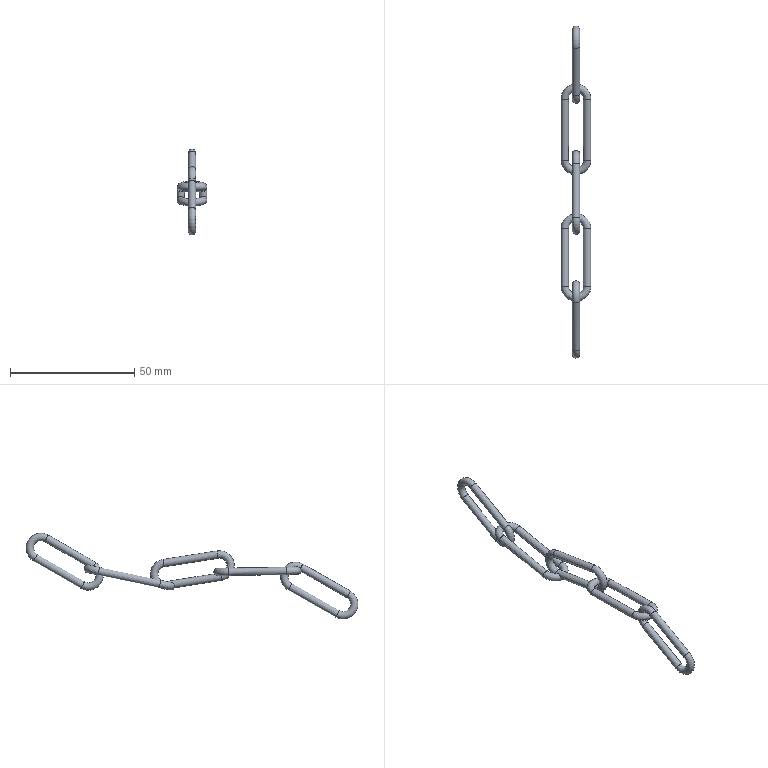Part | NX | features ACO1606-1-04.4 2 | 1 solid | 22 faces | box 12 x 133.567 x 34.55 mm | volume 2590 mm3 | cylinder 12 | torus 10 | commonest cylinder face diameters 3 x12
STEP:
#1=CARTESIAN_POINT('',(-1014.667,-666.313,-187.929));
#2=VERTEX_POINT('',#1);
#3=CARTESIAN_POINT('',(-1013.167,-665.571,-189.232));
#4=VERTEX_POINT('',#3);
#5=CARTESIAN_POINT('',(-1014.667,-665.571,-189.232));
#6=DIRECTION('',(0.,0.8691,0.4946));
#7=DIRECTION('',(1.,0.,0.));
#8=AXIS2_PLACEMENT_3D('',#5,#6,#7);
#9=CIRCLE('',#8,1.5);
#10=EDGE_CURVE('',#2,#4,#9,.T.);
#11=ORIENTED_EDGE('',*,*,#10,.T.);
#12=CARTESIAN_POINT('',(-1014.667,-664.829,-190.536));
#13=VERTEX_POINT('',#12);
#14=CARTESIAN_POINT('',(-1014.667,-665.571,-189.232));
#15=DIRECTION('',(0.,0.8691,0.4946));
#16=DIRECTION('',(1.,0.,0.));
#17=AXIS2_PLACEMENT_3D('',#14,#15,#16);
#18=CIRCLE('',#17,1.5);
#19=EDGE_CURVE('',#4,#13,#18,.T.);
#20=ORIENTED_EDGE('',*,*,#19,.T.);
#21=CARTESIAN_POINT('',(-1016.167,-665.571,-189.232));
#22=VERTEX_POINT('',#21);
#23=CARTESIAN_POINT('',(-1014.667,-665.571,-189.232));
#24=DIRECTION('',(0.,0.8691,0.4946));
#25=DIRECTION('',(1.,0.,0.));
#26=AXIS2_PLACEMENT_3D('',#23,#24,#25);
#27=CIRCLE('',#26,1.5);
#28=EDGE_CURVE('',#13,#22,#27,.T.);
#29=ORIENTED_EDGE('',*,*,#28,.T.);
#30=CARTESIAN_POINT('',(-1014.667,-665.571,-189.232));
#31=DIRECTION('',(0.,0.8691,0.4946));
#32=DIRECTION('',(1.,0.,0.));
#33=AXIS2_PLACEMENT_3D('',#30,#31,#32);
#34=CIRCLE('',#33,1.5);
#35=EDGE_CURVE('',#22,#2,#34,.T.);
#36=ORIENTED_EDGE('',*,*,#35,.T.);
#37=EDGE_LOOP('',(#11,#20,#29,#36));
#38=FACE_BOUND('',#37,.T.);
#39=CARTESIAN_POINT('',(-1013.333,-669.683,-182.007));
#40=VERTEX_POINT('',#39);
#41=CARTESIAN_POINT('',(-1014.667,-670.765,-180.107));
#42=VERTEX_POINT('',#41);
#43=CARTESIAN_POINT('',(-1014.667,-670.023,-181.41));
#44=DIRECTION('',(0.,-0.8691,-0.4946));
#45=DIRECTION('',(1.,0.,0.));
#46=AXIS2_PLACEMENT_3D('',#43,#44,#45);
#47=CIRCLE('',#46,1.5);
#48=EDGE_CURVE('',#40,#42,#47,.T.);
#49=ORIENTED_EDGE('',*,*,#48,.F.);
#50=CARTESIAN_POINT('',(-1016.001,-669.683,-182.007));
#51=VERTEX_POINT('',#50);
#52=CARTESIAN_POINT('',(-1013.333,-669.683,-182.007));
#53=CARTESIAN_POINT('',(-1013.251,-669.485,-181.709));
#54=CARTESIAN_POINT('',(-1013.206,-668.885,-181.238));
#55=CARTESIAN_POINT('',(-1013.224,-667.927,-181.234));
#56=CARTESIAN_POINT('',(-1013.353,-667.283,-181.603));
#57=CARTESIAN_POINT('',(-1013.736,-666.964,-182.19));
#58=CARTESIAN_POINT('',(-1014.663,-667.168,-182.548));
#59=CARTESIAN_POINT('',(-1015.587,-666.965,-182.199));
#60=CARTESIAN_POINT('',(-1015.978,-667.275,-181.609));
#61=CARTESIAN_POINT('',(-1016.11,-667.918,-181.235));
#62=CARTESIAN_POINT('',(-1016.128,-668.884,-181.237));
#63=CARTESIAN_POINT('',(-1016.084,-669.485,-181.709));
#64=CARTESIAN_POINT('',(-1016.001,-669.683,-182.007));
#65=B_SPLINE_CURVE_WITH_KNOTS('',3,(#52,#53,#54,#55,#56,#57,#58,#59,#60,#61,#62,#63,#64),.UNSPECIFIED.,.F.,.F.,(4,1,1,1,1,1,1,1,1,1,4),(0.,0.001085,0.002169,0.002711,0.003254,0.004338,0.005423,0.005965,0.006507,0.007592,0.008676),.UNSPECIFIED.);
#66=EDGE_CURVE('',#40,#51,#65,.T.);
#67=ORIENTED_EDGE('',*,*,#66,.T.);
#68=CARTESIAN_POINT('',(-1016.167,-670.023,-181.41));
#69=VERTEX_POINT('',#68);
#70=CARTESIAN_POINT('',(-1014.667,-670.023,-181.41));
#71=DIRECTION('',(0.,-0.8691,-0.4946));
#72=DIRECTION('',(1.,0.,0.));
#73=AXIS2_PLACEMENT_3D('',#70,#71,#72);
#74=CIRCLE('',#73,1.5);
#75=EDGE_CURVE('',#69,#51,#74,.T.);
#76=ORIENTED_EDGE('',*,*,#75,.F.);
#77=CARTESIAN_POINT('',(-1014.667,-670.023,-181.41));
#78=DIRECTION('',(0.,-0.8691,-0.4946));
#79=DIRECTION('',(1.,0.,0.));
#80=AXIS2_PLACEMENT_3D('',#77,#78,#79);
#81=CIRCLE('',#80,1.5);
#82=EDGE_CURVE('',#42,#69,#81,.T.);
#83=ORIENTED_EDGE('',*,*,#82,.F.);
#84=EDGE_LOOP('',(#49,#67,#76,#83));
#85=FACE_BOUND('',#84,.T.);
#86=CARTESIAN_POINT('',(-1014.667,-667.797,-185.321));
#87=DIRECTION('',(1.,0.,0.));
#88=DIRECTION('',(0.,0.,-1.));
#89=AXIS2_PLACEMENT_3D('',#86,#87,#88);
#90=TOROIDAL_SURFACE('',#89,4.5,1.5);
#91=ADVANCED_FACE('',(#38,#85),#90,.T.);
#92=CARTESIAN_POINT('',(-1016.001,-669.683,-182.007));
#93=CARTESIAN_POINT('',(-1015.928,-669.859,-182.27));
#94=CARTESIAN_POINT('',(-1015.636,-670.028,-182.868));
#95=CARTESIAN_POINT('',(-1014.667,-669.985,-183.25));
#96=CARTESIAN_POINT('',(-1013.698,-670.028,-182.868));
#97=CARTESIAN_POINT('',(-1013.406,-669.859,-182.27));
#98=CARTESIAN_POINT('',(-1013.333,-669.683,-182.007));
#99=B_SPLINE_CURVE_WITH_KNOTS('',3,(#92,#93,#94,#95,#96,#97,#98),.UNSPECIFIED.,.F.,.F.,(4,1,1,1,4),(-0.002944,-0.001984,-0.001024,-0.00006463,0.0008951),.UNSPECIFIED.);
#100=EDGE_CURVE('',#51,#40,#99,.T.);
#101=ORIENTED_EDGE('',*,*,#100,.T.);
#102=ORIENTED_EDGE('',*,*,#48,.T.);
#103=ORIENTED_EDGE('',*,*,#82,.T.);
#104=ORIENTED_EDGE('',*,*,#75,.T.);
#105=EDGE_LOOP('',(#101,#102,#103,#104));
#106=FACE_BOUND('',#105,.T.);
#107=CARTESIAN_POINT('',(-1013.167,-689.143,-192.292));
#108=VERTEX_POINT('',#107);
#109=CARTESIAN_POINT('',(-1014.667,-689.143,-192.292));
#110=DIRECTION('',(0.,-0.8691,-0.4946));
#111=DIRECTION('',(1.,0.,0.));
#112=AXIS2_PLACEMENT_3D('',#109,#110,#111);
#113=CIRCLE('',#112,1.5);
#114=EDGE_CURVE('',#108,#108,#113,.T.);
#115=ORIENTED_EDGE('',*,*,#114,.F.);
#116=EDGE_LOOP('',(#115));
#117=FACE_BOUND('',#116,.T.);
#118=CARTESIAN_POINT('',(-1014.667,-678.726,-186.364));
#119=DIRECTION('',(0.,0.8691,0.4946));
#120=DIRECTION('',(0.,0.4946,-0.8691));
#121=AXIS2_PLACEMENT_3D('',#118,#119,#120);
#122=CYLINDRICAL_SURFACE('',#121,1.5);
#123=ADVANCED_FACE('',(#106,#117),#122,.T.);
#124=CARTESIAN_POINT('',(-1013.167,-684.691,-200.114));
#125=VERTEX_POINT('',#124);
#126=CARTESIAN_POINT('',(-1014.667,-684.691,-200.114));
#127=DIRECTION('',(0.,0.8691,0.4946));
#128=DIRECTION('',(1.,0.,0.));
#129=AXIS2_PLACEMENT_3D('',#126,#127,#128);
#130=CIRCLE('',#129,1.5);
#131=EDGE_CURVE('',#125,#125,#130,.T.);
#132=ORIENTED_EDGE('',*,*,#131,.T.);
#133=EDGE_LOOP('',(#132));
#134=FACE_BOUND('',#133,.T.);
#135=ORIENTED_EDGE('',*,*,#19,.F.);
#136=ORIENTED_EDGE('',*,*,#10,.F.);
#137=ORIENTED_EDGE('',*,*,#35,.F.);
#138=ORIENTED_EDGE('',*,*,#28,.F.);
#139=EDGE_LOOP('',(#135,#136,#137,#138));
#140=FACE_BOUND('',#139,.T.);
#141=CARTESIAN_POINT('',(-1014.667,-675.988,-195.161));
#142=DIRECTION('',(0.,-0.8691,-0.4946));
#143=DIRECTION('',(0.,-0.4946,0.8691));
#144=AXIS2_PLACEMENT_3D('',#141,#142,#143);
#145=CYLINDRICAL_SURFACE('',#144,1.5);
#146=ADVANCED_FACE('',(#134,#140),#145,.T.);
#147=ORIENTED_EDGE('',*,*,#114,.T.);
#148=EDGE_LOOP('',(#147));
#149=FACE_BOUND('',#148,.T.);
#150=ORIENTED_EDGE('',*,*,#131,.F.);
#151=EDGE_LOOP('',(#150));
#152=FACE_BOUND('',#151,.T.);
#153=CARTESIAN_POINT('',(-1014.667,-686.917,-196.203));
#154=DIRECTION('',(1.,0.,0.));
#155=DIRECTION('',(0.,0.,-1.));
#156=AXIS2_PLACEMENT_3D('',#153,#154,#155);
#157=TOROIDAL_SURFACE('',#156,4.5,1.5);
#158=ADVANCED_FACE('',(#149,#152),#157,.T.);
#159=CARTESIAN_POINT('',(-1014.667,-563.854,-176.253));
#160=VERTEX_POINT('',#159);
#161=CARTESIAN_POINT('',(-1013.167,-563.106,-177.553));
#162=VERTEX_POINT('',#161);
#163=CARTESIAN_POINT('',(-1014.667,-563.106,-177.553));
#164=DIRECTION('',(0.,0.8667,0.4989));
#165=DIRECTION('',(1.,0.,0.));
#166=AXIS2_PLACEMENT_3D('',#163,#164,#165);
#167=CIRCLE('',#166,1.5);
#168=EDGE_CURVE('',#160,#162,#167,.T.);
#169=ORIENTED_EDGE('',*,*,#168,.T.);
#170=CARTESIAN_POINT('',(-1014.667,-562.357,-178.853));
#171=VERTEX_POINT('',#170);
#172=CARTESIAN_POINT('',(-1014.667,-563.106,-177.553));
#173=DIRECTION('',(0.,0.8667,0.4989));
#174=DIRECTION('',(1.,0.,0.));
#175=AXIS2_PLACEMENT_3D('',#172,#173,#174);
#176=CIRCLE('',#175,1.5);
#177=EDGE_CURVE('',#162,#171,#176,.T.);
#178=ORIENTED_EDGE('',*,*,#177,.T.);
#179=CARTESIAN_POINT('',(-1016.167,-563.106,-177.553));
#180=VERTEX_POINT('',#179);
#181=CARTESIAN_POINT('',(-1014.667,-563.106,-177.553));
#182=DIRECTION('',(0.,0.8667,0.4989));
#183=DIRECTION('',(1.,0.,0.));
#184=AXIS2_PLACEMENT_3D('',#181,#182,#183);
#185=CIRCLE('',#184,1.5);
#186=EDGE_CURVE('',#171,#180,#185,.T.);
#187=ORIENTED_EDGE('',*,*,#186,.T.);
#188=CARTESIAN_POINT('',(-1014.667,-563.106,-177.553));
#189=DIRECTION('',(0.,0.8667,0.4989));
#190=DIRECTION('',(1.,0.,0.));
#191=AXIS2_PLACEMENT_3D('',#188,#189,#190);
#192=CIRCLE('',#191,1.5);
#193=EDGE_CURVE('',#180,#160,#192,.T.);
#194=ORIENTED_EDGE('',*,*,#193,.T.);
#195=EDGE_LOOP('',(#169,#178,#187,#194));
#196=FACE_BOUND('',#195,.T.);
#197=CARTESIAN_POINT('',(-1014.667,-566.847,-171.053));
#198=VERTEX_POINT('',#197);
#199=CARTESIAN_POINT('',(-1014.667,-568.344,-168.453));
#200=VERTEX_POINT('',#199);
#201=CARTESIAN_POINT('',(-1014.667,-567.596,-169.753));
#202=DIRECTION('',(0.,-0.8667,-0.4989));
#203=DIRECTION('',(1.,0.,0.));
#204=AXIS2_PLACEMENT_3D('',#201,#202,#203);
#205=CIRCLE('',#204,1.5);
#206=EDGE_CURVE('',#198,#200,#205,.T.);
#207=ORIENTED_EDGE('',*,*,#206,.F.);
#208=CARTESIAN_POINT('',(-1016.167,-567.596,-169.753));
#209=VERTEX_POINT('',#208);
#210=CARTESIAN_POINT('',(-1014.667,-567.596,-169.753));
#211=DIRECTION('',(0.,-0.8667,-0.4989));
#212=DIRECTION('',(1.,0.,0.));
#213=AXIS2_PLACEMENT_3D('',#210,#211,#212);
#214=CIRCLE('',#213,1.5);
#215=EDGE_CURVE('',#209,#198,#214,.T.);
#216=ORIENTED_EDGE('',*,*,#215,.F.);
#217=CARTESIAN_POINT('',(-1014.667,-567.596,-169.753));
#218=DIRECTION('',(0.,-0.8667,-0.4989));
#219=DIRECTION('',(1.,0.,0.));
#220=AXIS2_PLACEMENT_3D('',#217,#218,#219);
#221=CIRCLE('',#220,1.5);
#222=EDGE_CURVE('',#200,#209,#221,.T.);
#223=ORIENTED_EDGE('',*,*,#222,.F.);
#224=EDGE_LOOP('',(#207,#216,#223));
#225=FACE_BOUND('',#224,.T.);
#226=CARTESIAN_POINT('',(-1014.667,-565.351,-173.653));
#227=DIRECTION('',(1.,0.,0.));
#228=DIRECTION('',(0.,0.,-1.));
#229=AXIS2_PLACEMENT_3D('',#226,#227,#228);
#230=TOROIDAL_SURFACE('',#229,4.5,1.5);
#231=ADVANCED_FACE('',(#196,#225),#230,.T.);
#232=CARTESIAN_POINT('',(-1014.667,-583.59,-180.692));
#233=VERTEX_POINT('',#232);
#234=CARTESIAN_POINT('',(-1015.729,-583.974,-180.542));
#235=CARTESIAN_POINT('',(-1014.667,-583.398,-180.766));
#236=CARTESIAN_POINT('',(-1013.607,-583.972,-180.542));
#237=CARTESIAN_POINT('',(-1013.39,-584.923,-180.625));
#238=CARTESIAN_POINT('',(-1013.422,-585.531,-181.052));
#239=CARTESIAN_POINT('',(-1013.648,-585.773,-181.529));
#240=CARTESIAN_POINT('',(-1014.123,-585.717,-181.843));
#241=CARTESIAN_POINT('',(-1014.667,-585.676,-181.929));
#242=CARTESIAN_POINT('',(-1015.209,-585.716,-181.843));
#243=CARTESIAN_POINT('',(-1015.684,-585.773,-181.531));
#244=CARTESIAN_POINT('',(-1015.912,-585.533,-181.055));
#245=CARTESIAN_POINT('',(-1015.944,-584.922,-180.624));
#246=CARTESIAN_POINT('',(-1015.729,-583.974,-180.542));
#247=CARTESIAN_POINT('',(-1014.667,-583.398,-180.766));
#248=CARTESIAN_POINT('',(-1013.607,-583.972,-180.542));
#249=B_SPLINE_CURVE_WITH_KNOTS('',3,(#234,#235,#236,#237,#238,#239,#240,#241,#242,#243,#244,#245,#246,#247,#248),.UNSPECIFIED.,.T.,.F.,(1,1,1,1,1,1,1,1,1,1,1,1,1,1,1,1,1,1,1),(-0.002704,-0.002163,-0.001082,0.,0.001082,0.002163,0.002704,0.003245,0.003786,0.004327,0.004867,0.005408,0.005949,0.00649,0.007572,0.008653,0.009735,0.01082,0.01136),.UNSPECIFIED.);
#250=EDGE_CURVE('',#233,#233,#249,.T.);
#251=ORIENTED_EDGE('',*,*,#250,.F.);
#252=EDGE_LOOP('',(#251));
#253=FACE_BOUND('',#252,.T.);
#254=ORIENTED_EDGE('',*,*,#206,.T.);
#255=ORIENTED_EDGE('',*,*,#222,.T.);
#256=ORIENTED_EDGE('',*,*,#215,.T.);
#257=EDGE_LOOP('',(#254,#255,#256));
#258=FACE_BOUND('',#257,.T.);
#259=CARTESIAN_POINT('',(-1013.167,-586.662,-180.729));
#260=VERTEX_POINT('',#259);
#261=CARTESIAN_POINT('',(-1014.667,-586.662,-180.729));
#262=DIRECTION('',(0.,-0.8667,-0.4989));
#263=DIRECTION('',(1.,0.,0.));
#264=AXIS2_PLACEMENT_3D('',#261,#262,#263);
#265=CIRCLE('',#264,1.5);
#266=EDGE_CURVE('',#260,#260,#265,.T.);
#267=ORIENTED_EDGE('',*,*,#266,.F.);
#268=EDGE_LOOP('',(#267));
#269=FACE_BOUND('',#268,.T.);
#270=CARTESIAN_POINT('',(-1014.667,-576.298,-174.763));
#271=DIRECTION('',(0.,0.8667,0.4989));
#272=DIRECTION('',(0.,0.4989,-0.8667));
#273=AXIS2_PLACEMENT_3D('',#270,#271,#272);
#274=CYLINDRICAL_SURFACE('',#273,1.5);
#275=ADVANCED_FACE('',(#253,#258,#269),#274,.T.);
#276=CARTESIAN_POINT('',(-1013.167,-582.172,-188.529));
#277=VERTEX_POINT('',#276);
#278=CARTESIAN_POINT('',(-1014.667,-582.172,-188.529));
#279=DIRECTION('',(0.,0.8667,0.4989));
#280=DIRECTION('',(1.,0.,0.));
#281=AXIS2_PLACEMENT_3D('',#278,#279,#280);
#282=CIRCLE('',#281,1.5);
#283=EDGE_CURVE('',#277,#277,#282,.T.);
#284=ORIENTED_EDGE('',*,*,#283,.T.);
#285=EDGE_LOOP('',(#284));
#286=FACE_BOUND('',#285,.T.);
#287=ORIENTED_EDGE('',*,*,#177,.F.);
#288=ORIENTED_EDGE('',*,*,#168,.F.);
#289=ORIENTED_EDGE('',*,*,#193,.F.);
#290=ORIENTED_EDGE('',*,*,#186,.F.);
#291=EDGE_LOOP('',(#287,#288,#289,#290));
#292=FACE_BOUND('',#291,.T.);
#293=CARTESIAN_POINT('',(-1014.667,-573.47,-183.52));
#294=DIRECTION('',(0.,-0.8667,-0.4989));
#295=DIRECTION('',(0.,-0.4989,0.8667));
#296=AXIS2_PLACEMENT_3D('',#293,#294,#295);
#297=CYLINDRICAL_SURFACE('',#296,1.5);
#298=ADVANCED_FACE('',(#286,#292),#297,.T.);
#299=ORIENTED_EDGE('',*,*,#266,.T.);
#300=EDGE_LOOP('',(#299));
#301=FACE_BOUND('',#300,.T.);
#302=ORIENTED_EDGE('',*,*,#283,.F.);
#303=EDGE_LOOP('',(#302));
#304=FACE_BOUND('',#303,.T.);
#305=CARTESIAN_POINT('',(-1014.667,-584.417,-184.629));
#306=DIRECTION('',(1.,0.,0.));
#307=DIRECTION('',(0.,0.,-1.));
#308=AXIS2_PLACEMENT_3D('',#305,#306,#307);
#309=TOROIDAL_SURFACE('',#308,4.5,1.5);
#310=ADVANCED_FACE('',(#301,#304),#309,.T.);
#311=CARTESIAN_POINT('',(-1008.667,-588.604,-182.98));
#312=VERTEX_POINT('',#311);
#313=CARTESIAN_POINT('',(-1010.167,-588.604,-182.98));
#314=DIRECTION('',(0.,-0.979,-0.2038));
#315=DIRECTION('',(1.,0.,0.));
#316=AXIS2_PLACEMENT_3D('',#313,#314,#315);
#317=CIRCLE('',#316,1.5);
#318=EDGE_CURVE('',#312,#312,#317,.T.);
#319=ORIENTED_EDGE('',*,*,#318,.F.);
#320=EDGE_LOOP('',(#319));
#321=FACE_BOUND('',#320,.T.);
#322=CARTESIAN_POINT('',(-1017.667,-588.604,-182.98));
#323=VERTEX_POINT('',#322);
#324=CARTESIAN_POINT('',(-1019.167,-588.604,-182.98));
#325=DIRECTION('',(0.,0.979,0.2038));
#326=DIRECTION('',(1.,0.,0.));
#327=AXIS2_PLACEMENT_3D('',#324,#325,#326);
#328=CIRCLE('',#327,1.5);
#329=EDGE_CURVE('',#323,#323,#328,.T.);
#330=ORIENTED_EDGE('',*,*,#329,.T.);
#331=EDGE_LOOP('',(#330));
#332=FACE_BOUND('',#331,.T.);
#333=ORIENTED_EDGE('',*,*,#250,.T.);
#334=EDGE_LOOP('',(#333));
#335=FACE_BOUND('',#334,.T.);
#336=CARTESIAN_POINT('',(-1014.667,-588.604,-182.98));
#337=DIRECTION('',(0.,-0.2038,0.979));
#338=DIRECTION('',(0.,0.979,0.2038));
#339=AXIS2_PLACEMENT_3D('',#336,#337,#338);
#340=TOROIDAL_SURFACE('',#339,4.5,1.5);
#341=ADVANCED_FACE('',(#321,#332,#335),#340,.T.);
#342=CARTESIAN_POINT('',(-1017.667,-613.277,-188.116));
#343=VERTEX_POINT('',#342);
#344=CARTESIAN_POINT('',(-1019.167,-613.277,-188.116));
#345=DIRECTION('',(0.,0.979,0.2038));
#346=DIRECTION('',(1.,0.,0.));
#347=AXIS2_PLACEMENT_3D('',#344,#345,#346);
#348=CIRCLE('',#347,1.5);
#349=EDGE_CURVE('',#343,#343,#348,.T.);
#350=ORIENTED_EDGE('',*,*,#349,.T.);
#351=EDGE_LOOP('',(#350));
#352=FACE_BOUND('',#351,.T.);
#353=ORIENTED_EDGE('',*,*,#329,.F.);
#354=EDGE_LOOP('',(#353));
#355=FACE_BOUND('',#354,.T.);
#356=CARTESIAN_POINT('',(-1019.167,-600.94,-185.548));
#357=DIRECTION('',(0.,-0.979,-0.2038));
#358=DIRECTION('',(0.,-0.2038,0.979));
#359=AXIS2_PLACEMENT_3D('',#356,#357,#358);
#360=CYLINDRICAL_SURFACE('',#359,1.5);
#361=ADVANCED_FACE('',(#352,#355),#360,.T.);
#362=ORIENTED_EDGE('',*,*,#318,.T.);
#363=EDGE_LOOP('',(#362));
#364=FACE_BOUND('',#363,.T.);
#365=CARTESIAN_POINT('',(-1008.667,-613.277,-188.116));
#366=VERTEX_POINT('',#365);
#367=CARTESIAN_POINT('',(-1010.167,-613.277,-188.116));
#368=DIRECTION('',(0.,-0.979,-0.2038));
#369=DIRECTION('',(1.,0.,0.));
#370=AXIS2_PLACEMENT_3D('',#367,#368,#369);
#371=CIRCLE('',#370,1.5);
#372=EDGE_CURVE('',#366,#366,#371,.T.);
#373=ORIENTED_EDGE('',*,*,#372,.F.);
#374=EDGE_LOOP('',(#373));
#375=FACE_BOUND('',#374,.T.);
#376=CARTESIAN_POINT('',(-1010.167,-600.94,-185.548));
#377=DIRECTION('',(0.,-0.979,-0.2038));
#378=DIRECTION('',(0.,-0.2038,0.979));
#379=AXIS2_PLACEMENT_3D('',#376,#377,#378);
#380=CYLINDRICAL_SURFACE('',#379,1.5);
#381=ADVANCED_FACE('',(#364,#375),#380,.T.);
#382=ORIENTED_EDGE('',*,*,#349,.F.);
#383=EDGE_LOOP('',(#382));
#384=FACE_BOUND('',#383,.T.);
#385=CARTESIAN_POINT('',(-1013.167,-615.821,-188.645));
#386=VERTEX_POINT('',#385);
#387=CARTESIAN_POINT('',(-1013.167,-615.823,-188.637));
#388=VERTEX_POINT('',#387);
#389=CARTESIAN_POINT('',(-1013.167,-615.821,-188.645));
#390=CARTESIAN_POINT('',(-1013.167,-615.821,-188.643));
#391=CARTESIAN_POINT('',(-1013.167,-615.822,-188.64));
#392=CARTESIAN_POINT('',(-1013.167,-615.823,-188.637));
#393=B_SPLINE_CURVE_WITH_KNOTS('',3,(#389,#390,#391,#392),.UNSPECIFIED.,.F.,.F.,(4,4),(0.,1.),.PIECEWISE_BEZIER_KNOTS.);
#394=EDGE_CURVE('',#386,#388,#393,.T.);
#395=ORIENTED_EDGE('',*,*,#394,.T.);
#396=CARTESIAN_POINT('',(-1013.228,-616.052,-188.182));
#397=VERTEX_POINT('',#396);
#398=CARTESIAN_POINT('',(-1013.167,-615.823,-188.637));
#399=CARTESIAN_POINT('',(-1013.167,-615.859,-188.466));
#400=CARTESIAN_POINT('',(-1013.194,-615.944,-188.314));
#401=CARTESIAN_POINT('',(-1013.228,-616.052,-188.182));
#402=B_SPLINE_CURVE_WITH_KNOTS('',3,(#398,#399,#400,#401),.UNSPECIFIED.,.F.,.F.,(4,4),(0.,0.0005142),.UNSPECIFIED.);
#403=EDGE_CURVE('',#388,#397,#402,.T.);
#404=ORIENTED_EDGE('',*,*,#403,.T.);
#405=CARTESIAN_POINT('',(-1016.106,-616.052,-188.182));
#406=VERTEX_POINT('',#405);
#407=CARTESIAN_POINT('',(-1016.106,-616.052,-188.182));
#408=CARTESIAN_POINT('',(-1016.016,-616.342,-187.825));
#409=CARTESIAN_POINT('',(-1015.703,-617.189,-187.342));
#410=CARTESIAN_POINT('',(-1016.248,-618.634,-187.689));
#411=CARTESIAN_POINT('',(-1016.071,-619.192,-189.171));
#412=CARTESIAN_POINT('',(-1014.667,-618.976,-189.895));
#413=CARTESIAN_POINT('',(-1013.264,-619.192,-189.172));
#414=CARTESIAN_POINT('',(-1013.085,-618.635,-187.691));
#415=CARTESIAN_POINT('',(-1013.632,-617.192,-187.341));
#416=CARTESIAN_POINT('',(-1013.318,-616.343,-187.824));
#417=CARTESIAN_POINT('',(-1013.228,-616.052,-188.182));
#418=B_SPLINE_CURVE_WITH_KNOTS('',3,(#407,#408,#409,#410,#411,#412,#413,#414,#415,#416,#417),.UNSPECIFIED.,.F.,.F.,(4,1,1,1,1,1,1,1,4),(0.,0.001383,0.002766,0.00415,0.005533,0.006916,0.008299,0.009683,0.01107),.UNSPECIFIED.);
#419=EDGE_CURVE('',#406,#397,#418,.T.);
#420=ORIENTED_EDGE('',*,*,#419,.F.);
#421=CARTESIAN_POINT('',(-1016.167,-615.823,-188.637));
#422=VERTEX_POINT('',#421);
#423=CARTESIAN_POINT('',(-1016.167,-615.823,-188.637));
#424=CARTESIAN_POINT('',(-1016.167,-615.859,-188.466));
#425=CARTESIAN_POINT('',(-1016.14,-615.944,-188.314));
#426=CARTESIAN_POINT('',(-1016.106,-616.052,-188.182));
#427=B_SPLINE_CURVE_WITH_KNOTS('',3,(#423,#424,#425,#426),.UNSPECIFIED.,.F.,.F.,(4,4),(0.,0.0005142),.UNSPECIFIED.);
#428=EDGE_CURVE('',#406,#422,#427,.F.);
#429=ORIENTED_EDGE('',*,*,#428,.T.);
#430=CARTESIAN_POINT('',(-1016.167,-615.821,-188.645));
#431=VERTEX_POINT('',#430);
#432=CARTESIAN_POINT('',(-1016.167,-615.821,-188.645));
#433=CARTESIAN_POINT('',(-1016.167,-615.821,-188.643));
#434=CARTESIAN_POINT('',(-1016.167,-615.822,-188.64));
#435=CARTESIAN_POINT('',(-1016.167,-615.823,-188.637));
#436=B_SPLINE_CURVE_WITH_KNOTS('',3,(#432,#433,#434,#435),.UNSPECIFIED.,.F.,.F.,(4,4),(0.,1.),.PIECEWISE_BEZIER_KNOTS.);
#437=EDGE_CURVE('',#422,#431,#436,.F.);
#438=ORIENTED_EDGE('',*,*,#437,.T.);
#439=CARTESIAN_POINT('',(-1015.523,-616.311,-189.817));
#440=VERTEX_POINT('',#439);
#441=CARTESIAN_POINT('',(-1016.167,-615.821,-188.645));
#442=CARTESIAN_POINT('',(-1016.164,-615.718,-189.147));
#443=CARTESIAN_POINT('',(-1015.907,-616.074,-189.584));
#444=CARTESIAN_POINT('',(-1015.523,-616.311,-189.817));
#445=B_SPLINE_CURVE_WITH_KNOTS('',3,(#441,#442,#443,#444),.UNSPECIFIED.,.F.,.F.,(4,4),(0.,0.001512),.UNSPECIFIED.);
#446=EDGE_CURVE('',#431,#440,#445,.T.);
#447=ORIENTED_EDGE('',*,*,#446,.T.);
#448=CARTESIAN_POINT('',(-1013.811,-616.311,-189.817));
#449=VERTEX_POINT('',#448);
#450=CARTESIAN_POINT('',(-1015.523,-616.311,-189.817));
#451=CARTESIAN_POINT('',(-1015.283,-616.459,-189.962));
#452=CARTESIAN_POINT('',(-1014.666,-616.694,-190.13));
#453=CARTESIAN_POINT('',(-1014.051,-616.459,-189.962));
#454=CARTESIAN_POINT('',(-1013.811,-616.311,-189.817));
#455=B_SPLINE_CURVE_WITH_KNOTS('',3,(#450,#451,#452,#453,#454),.UNSPECIFIED.,.F.,.F.,(4,1,4),(-0.0009365,0.000000498,0.0009375),.UNSPECIFIED.);
#456=EDGE_CURVE('',#440,#449,#455,.T.);
#457=ORIENTED_EDGE('',*,*,#456,.T.);
#458=CARTESIAN_POINT('',(-1013.167,-615.821,-188.645));
#459=CARTESIAN_POINT('',(-1013.17,-615.718,-189.147));
#460=CARTESIAN_POINT('',(-1013.427,-616.074,-189.584));
#461=CARTESIAN_POINT('',(-1013.811,-616.311,-189.817));
#462=B_SPLINE_CURVE_WITH_KNOTS('',3,(#458,#459,#460,#461),.UNSPECIFIED.,.F.,.F.,(4,4),(0.,0.001512),.UNSPECIFIED.);
#463=EDGE_CURVE('',#449,#386,#462,.F.);
#464=ORIENTED_EDGE('',*,*,#463,.T.);
#465=EDGE_LOOP('',(#395,#404,#420,#429,#438,#447,#457,#464));
#466=FACE_BOUND('',#465,.T.);
#467=ORIENTED_EDGE('',*,*,#372,.T.);
#468=EDGE_LOOP('',(#467));
#469=FACE_BOUND('',#468,.T.);
#470=CARTESIAN_POINT('',(-1014.667,-613.277,-188.116));
#471=DIRECTION('',(0.,-0.2038,0.979));
#472=DIRECTION('',(0.,0.979,0.2038));
#473=AXIS2_PLACEMENT_3D('',#470,#471,#472);
#474=TOROIDAL_SURFACE('',#473,4.5,1.5);
#475=ADVANCED_FACE('',(#384,#466,#469),#474,.T.);
#476=CARTESIAN_POINT('',(-1014.667,-616.353,-190.081));
#477=VERTEX_POINT('',#476);
#478=CARTESIAN_POINT('',(-1014.667,-616.118,-188.6));
#479=DIRECTION('',(0.,0.9877,-0.1566));
#480=DIRECTION('',(1.,0.,0.));
#481=AXIS2_PLACEMENT_3D('',#478,#479,#480);
#482=CIRCLE('',#481,1.5);
#483=EDGE_CURVE('',#477,#440,#482,.T.);
#484=ORIENTED_EDGE('',*,*,#483,.T.);
#485=ORIENTED_EDGE('',*,*,#446,.F.);
#486=ORIENTED_EDGE('',*,*,#437,.F.);
#487=ORIENTED_EDGE('',*,*,#428,.F.);
#488=CARTESIAN_POINT('',(-1014.667,-616.118,-188.6));
#489=DIRECTION('',(0.,0.9877,-0.1566));
#490=DIRECTION('',(1.,0.,0.));
#491=AXIS2_PLACEMENT_3D('',#488,#489,#490);
#492=CIRCLE('',#491,1.5);
#493=EDGE_CURVE('',#406,#397,#492,.T.);
#494=ORIENTED_EDGE('',*,*,#493,.T.);
#495=ORIENTED_EDGE('',*,*,#403,.F.);
#496=ORIENTED_EDGE('',*,*,#394,.F.);
#497=ORIENTED_EDGE('',*,*,#463,.F.);
#498=CARTESIAN_POINT('',(-1014.667,-616.118,-188.6));
#499=DIRECTION('',(0.,0.9877,-0.1566));
#500=DIRECTION('',(1.,0.,0.));
#501=AXIS2_PLACEMENT_3D('',#498,#499,#500);
#502=CIRCLE('',#501,1.5);
#503=EDGE_CURVE('',#449,#477,#502,.T.);
#504=ORIENTED_EDGE('',*,*,#503,.T.);
#505=EDGE_LOOP('',(#484,#485,#486,#487,#494,#495,#496,#497,#504));
#506=FACE_BOUND('',#505,.T.);
#507=CARTESIAN_POINT('',(-1014.667,-614.944,-181.192));
#508=VERTEX_POINT('',#507);
#509=CARTESIAN_POINT('',(-1014.667,-614.474,-178.229));
#510=VERTEX_POINT('',#509);
#511=CARTESIAN_POINT('',(-1014.667,-614.709,-179.711));
#512=DIRECTION('',(0.,-0.9877,0.1566));
#513=DIRECTION('',(1.,0.,0.));
#514=AXIS2_PLACEMENT_3D('',#511,#512,#513);
#515=CIRCLE('',#514,1.5);
#516=EDGE_CURVE('',#508,#510,#515,.T.);
#517=ORIENTED_EDGE('',*,*,#516,.F.);
#518=CARTESIAN_POINT('',(-1016.167,-614.709,-179.711));
#519=VERTEX_POINT('',#518);
#520=CARTESIAN_POINT('',(-1014.667,-614.709,-179.711));
#521=DIRECTION('',(0.,-0.9877,0.1566));
#522=DIRECTION('',(1.,0.,0.));
#523=AXIS2_PLACEMENT_3D('',#520,#521,#522);
#524=CIRCLE('',#523,1.5);
#525=EDGE_CURVE('',#519,#508,#524,.T.);
#526=ORIENTED_EDGE('',*,*,#525,.F.);
#527=CARTESIAN_POINT('',(-1014.667,-614.709,-179.711));
#528=DIRECTION('',(0.,-0.9877,0.1566));
#529=DIRECTION('',(1.,0.,0.));
#530=AXIS2_PLACEMENT_3D('',#527,#528,#529);
#531=CIRCLE('',#530,1.5);
#532=EDGE_CURVE('',#510,#519,#531,.T.);
#533=ORIENTED_EDGE('',*,*,#532,.F.);
#534=EDGE_LOOP('',(#517,#526,#533));
#535=FACE_BOUND('',#534,.T.);
#536=CARTESIAN_POINT('',(-1014.667,-615.413,-184.155));
#537=DIRECTION('',(1.,0.,0.));
#538=DIRECTION('',(0.,0.,-1.));
#539=AXIS2_PLACEMENT_3D('',#536,#537,#538);
#540=TOROIDAL_SURFACE('',#539,4.5,1.5);
#541=ADVANCED_FACE('',(#506,#535),#540,.T.);
#542=CARTESIAN_POINT('',(-1013.435,-637.713,-184.31));
#543=VERTEX_POINT('',#542);
#544=CARTESIAN_POINT('',(-1015.899,-637.713,-184.31));
#545=VERTEX_POINT('',#544);
#546=CARTESIAN_POINT('',(-1014.667,-637.847,-185.154));
#547=DIRECTION('',(0.,0.9877,-0.1566));
#548=DIRECTION('',(1.,0.,0.));
#549=AXIS2_PLACEMENT_3D('',#546,#547,#548);
#550=CIRCLE('',#549,1.5);
#551=EDGE_CURVE('',#543,#545,#550,.T.);
#552=ORIENTED_EDGE('',*,*,#551,.T.);
#553=CARTESIAN_POINT('',(-1015.899,-637.713,-184.31));
#554=CARTESIAN_POINT('',(-1016.038,-637.542,-184.539));
#555=CARTESIAN_POINT('',(-1016.095,-636.953,-184.86));
#556=CARTESIAN_POINT('',(-1016.042,-635.98,-184.778));
#557=CARTESIAN_POINT('',(-1015.611,-635.238,-184.276));
#558=CARTESIAN_POINT('',(-1014.67,-635.006,-183.974));
#559=CARTESIAN_POINT('',(-1013.727,-635.234,-184.273));
#560=CARTESIAN_POINT('',(-1013.292,-635.979,-184.778));
#561=CARTESIAN_POINT('',(-1013.239,-636.952,-184.86));
#562=CARTESIAN_POINT('',(-1013.296,-637.542,-184.539));
#563=CARTESIAN_POINT('',(-1013.435,-637.713,-184.31));
#564=B_SPLINE_CURVE_WITH_KNOTS('',3,(#553,#554,#555,#556,#557,#558,#559,#560,#561,#562,#563),.UNSPECIFIED.,.F.,.F.,(4,1,1,1,1,1,1,1,4),(0.,0.0009385,0.001877,0.002816,0.003754,0.004693,0.005631,0.00657,0.007508),.UNSPECIFIED.);
#565=EDGE_CURVE('',#545,#543,#564,.T.);
#566=ORIENTED_EDGE('',*,*,#565,.T.);
#567=EDGE_LOOP('',(#552,#566));
#568=FACE_BOUND('',#567,.T.);
#569=ORIENTED_EDGE('',*,*,#493,.F.);
#570=ORIENTED_EDGE('',*,*,#419,.T.);
#571=EDGE_LOOP('',(#569,#570));
#572=FACE_BOUND('',#571,.T.);
#573=CARTESIAN_POINT('',(-1014.667,-626.278,-186.989));
#574=DIRECTION('',(0.,-0.9877,0.1566));
#575=DIRECTION('',(0.,0.1566,0.9877));
#576=AXIS2_PLACEMENT_3D('',#573,#574,#575);
#577=CYLINDRICAL_SURFACE('',#576,1.5);
#578=ADVANCED_FACE('',(#568,#572),#577,.T.);
#579=ORIENTED_EDGE('',*,*,#503,.F.);
#580=ORIENTED_EDGE('',*,*,#456,.F.);
#581=ORIENTED_EDGE('',*,*,#483,.F.);
#582=EDGE_LOOP('',(#579,#580,#581));
#583=FACE_BOUND('',#582,.T.);
#584=CARTESIAN_POINT('',(-1014.667,-626.278,-186.989));
#585=DIRECTION('',(0.,-0.9877,0.1566));
#586=DIRECTION('',(0.,0.1566,0.9877));
#587=AXIS2_PLACEMENT_3D('',#584,#585,#586);
#588=CYLINDRICAL_SURFACE('',#587,1.5);
#589=ADVANCED_FACE('',(#583),#588,.T.);
#590=ORIENTED_EDGE('',*,*,#532,.T.);
#591=ORIENTED_EDGE('',*,*,#525,.T.);
#592=ORIENTED_EDGE('',*,*,#516,.T.);
#593=EDGE_LOOP('',(#590,#591,#592));
#594=FACE_BOUND('',#593,.T.);
#595=CARTESIAN_POINT('',(-1013.167,-636.437,-176.265));
#596=VERTEX_POINT('',#595);
#597=CARTESIAN_POINT('',(-1014.667,-636.672,-177.747));
#598=VERTEX_POINT('',#597);
#599=CARTESIAN_POINT('',(-1014.667,-636.437,-176.265));
#600=DIRECTION('',(0.,-0.9877,0.1566));
#601=DIRECTION('',(1.,0.,0.));
#602=AXIS2_PLACEMENT_3D('',#599,#600,#601);
#603=CIRCLE('',#602,1.5);
#604=EDGE_CURVE('',#596,#598,#603,.T.);
#605=ORIENTED_EDGE('',*,*,#604,.F.);
#606=CARTESIAN_POINT('',(-1014.667,-636.437,-176.265));
#607=DIRECTION('',(0.,-0.9877,0.1566));
#608=DIRECTION('',(1.,0.,0.));
#609=AXIS2_PLACEMENT_3D('',#606,#607,#608);
#610=CIRCLE('',#609,1.5);
#611=EDGE_CURVE('',#598,#596,#610,.T.);
#612=ORIENTED_EDGE('',*,*,#611,.F.);
#613=EDGE_LOOP('',(#605,#612));
#614=FACE_BOUND('',#613,.T.);
#615=CARTESIAN_POINT('',(-1014.667,-626.278,-177.876));
#616=DIRECTION('',(0.,-0.9877,0.1566));
#617=DIRECTION('',(0.,0.1566,0.9877));
#618=AXIS2_PLACEMENT_3D('',#615,#616,#617);
#619=CYLINDRICAL_SURFACE('',#618,1.5);
#620=ADVANCED_FACE('',(#594,#614),#619,.T.);
#621=ORIENTED_EDGE('',*,*,#604,.T.);
#622=ORIENTED_EDGE('',*,*,#611,.T.);
#623=EDGE_LOOP('',(#621,#622));
#624=FACE_BOUND('',#623,.T.);
#625=CARTESIAN_POINT('',(-1015.899,-637.713,-184.31));
#626=CARTESIAN_POINT('',(-1015.678,-637.984,-183.944));
#627=CARTESIAN_POINT('',(-1014.665,-637.687,-183.314));
#628=CARTESIAN_POINT('',(-1013.657,-637.985,-183.943));
#629=CARTESIAN_POINT('',(-1013.435,-637.713,-184.31));
#630=B_SPLINE_CURVE_WITH_KNOTS('',3,(#625,#626,#627,#628,#629),.UNSPECIFIED.,.F.,.F.,(4,1,4),(0.,0.001498,0.002997),.UNSPECIFIED.);
#631=EDGE_CURVE('',#545,#543,#630,.T.);
#632=ORIENTED_EDGE('',*,*,#631,.F.);
#633=ORIENTED_EDGE('',*,*,#551,.F.);
#634=EDGE_LOOP('',(#632,#633));
#635=FACE_BOUND('',#634,.T.);
#636=CARTESIAN_POINT('',(-1014.667,-637.142,-180.71));
#637=DIRECTION('',(1.,0.,0.));
#638=DIRECTION('',(0.,0.,-1.));
#639=AXIS2_PLACEMENT_3D('',#636,#637,#638);
#640=TOROIDAL_SURFACE('',#639,4.5,1.5);
#641=ADVANCED_FACE('',(#624,#635),#640,.T.);
#642=CARTESIAN_POINT('',(-1008.667,-640.87,-183.23));
#643=VERTEX_POINT('',#642);
#644=CARTESIAN_POINT('',(-1010.167,-640.87,-183.23));
#645=DIRECTION('',(0.,0.9999,-0.01692));
#646=DIRECTION('',(1.,0.,0.));
#647=AXIS2_PLACEMENT_3D('',#644,#645,#646);
#648=CIRCLE('',#647,1.5);
#649=EDGE_CURVE('',#643,#643,#648,.T.);
#650=ORIENTED_EDGE('',*,*,#649,.T.);
#651=EDGE_LOOP('',(#650));
#652=FACE_BOUND('',#651,.T.);
#653=CARTESIAN_POINT('',(-1017.667,-640.87,-183.23));
#654=VERTEX_POINT('',#653);
#655=CARTESIAN_POINT('',(-1019.167,-640.87,-183.23));
#656=DIRECTION('',(0.,-0.9999,0.01692));
#657=DIRECTION('',(1.,0.,0.));
#658=AXIS2_PLACEMENT_3D('',#655,#656,#657);
#659=CIRCLE('',#658,1.5);
#660=EDGE_CURVE('',#654,#654,#659,.T.);
#661=ORIENTED_EDGE('',*,*,#660,.F.);
#662=EDGE_LOOP('',(#661));
#663=FACE_BOUND('',#662,.T.);
#664=ORIENTED_EDGE('',*,*,#565,.F.);
#665=ORIENTED_EDGE('',*,*,#631,.T.);
#666=EDGE_LOOP('',(#664,#665));
#667=FACE_BOUND('',#666,.T.);
#668=CARTESIAN_POINT('',(-1014.667,-640.87,-183.23));
#669=DIRECTION('',(0.,0.01692,0.9999));
#670=DIRECTION('',(0.,0.9999,-0.01692));
#671=AXIS2_PLACEMENT_3D('',#668,#669,#670);
#672=TOROIDAL_SURFACE('',#671,4.5,1.5);
#673=ADVANCED_FACE('',(#652,#663,#667),#672,.T.);
#674=CARTESIAN_POINT('',(-1017.667,-664.045,-182.838));
#675=VERTEX_POINT('',#674);
#676=CARTESIAN_POINT('',(-1019.167,-664.045,-182.838));
#677=DIRECTION('',(0.,-0.9999,0.01692));
#678=DIRECTION('',(1.,0.,0.));
#679=AXIS2_PLACEMENT_3D('',#676,#677,#678);
#680=CIRCLE('',#679,1.5);
#681=EDGE_CURVE('',#675,#675,#680,.T.);
#682=ORIENTED_EDGE('',*,*,#681,.F.);
#683=EDGE_LOOP('',(#682));
#684=FACE_BOUND('',#683,.T.);
#685=ORIENTED_EDGE('',*,*,#660,.T.);
#686=EDGE_LOOP('',(#685));
#687=FACE_BOUND('',#686,.T.);
#688=CARTESIAN_POINT('',(-1019.167,-652.457,-183.034));
#689=DIRECTION('',(0.,0.9999,-0.01692));
#690=DIRECTION('',(0.,-0.01692,-0.9999));
#691=AXIS2_PLACEMENT_3D('',#688,#689,#690);
#692=CYLINDRICAL_SURFACE('',#691,1.5);
#693=ADVANCED_FACE('',(#684,#687),#692,.T.);
#694=ORIENTED_EDGE('',*,*,#649,.F.);
#695=EDGE_LOOP('',(#694));
#696=FACE_BOUND('',#695,.T.);
#697=CARTESIAN_POINT('',(-1008.667,-664.045,-182.838));
#698=VERTEX_POINT('',#697);
#699=CARTESIAN_POINT('',(-1010.167,-664.045,-182.838));
#700=DIRECTION('',(0.,0.9999,-0.01692));
#701=DIRECTION('',(1.,0.,0.));
#702=AXIS2_PLACEMENT_3D('',#699,#700,#701);
#703=CIRCLE('',#702,1.5);
#704=EDGE_CURVE('',#698,#698,#703,.T.);
#705=ORIENTED_EDGE('',*,*,#704,.T.);
#706=EDGE_LOOP('',(#705));
#707=FACE_BOUND('',#706,.T.);
#708=CARTESIAN_POINT('',(-1010.167,-652.457,-183.034));
#709=DIRECTION('',(0.,-0.9999,0.01692));
#710=DIRECTION('',(0.,0.01692,0.9999));
#711=AXIS2_PLACEMENT_3D('',#708,#709,#710);
#712=CYLINDRICAL_SURFACE('',#711,1.5);
#713=ADVANCED_FACE('',(#696,#707),#712,.T.);
#714=ORIENTED_EDGE('',*,*,#681,.T.);
#715=EDGE_LOOP('',(#714));
#716=FACE_BOUND('',#715,.T.);
#717=ORIENTED_EDGE('',*,*,#66,.F.);
#718=ORIENTED_EDGE('',*,*,#100,.F.);
#719=EDGE_LOOP('',(#717,#718));
#720=FACE_BOUND('',#719,.T.);
#721=ORIENTED_EDGE('',*,*,#704,.F.);
#722=EDGE_LOOP('',(#721));
#723=FACE_BOUND('',#722,.T.);
#724=CARTESIAN_POINT('',(-1014.667,-664.045,-182.838));
#725=DIRECTION('',(0.,0.01692,0.9999));
#726=DIRECTION('',(0.,0.9999,-0.01692));
#727=AXIS2_PLACEMENT_3D('',#724,#725,#726);
#728=TOROIDAL_SURFACE('',#727,4.5,1.5);
#729=ADVANCED_FACE('',(#716,#720,#723),#728,.T.);
#730=CLOSED_SHELL('',(#91,#123,#146,#158,#231,#275,#298,#310,#341,#361,#381,#475,#541,#578,#589,#620,#641,#673,#693,#713,#729));
#731=MANIFOLD_SOLID_BREP('',#730);
#732=(LENGTH_UNIT()NAMED_UNIT(*)SI_UNIT(.MILLI.,.METRE.));
#733=UNCERTAINTY_MEASURE_WITH_UNIT(LENGTH_MEASURE(0.0508),#732,'','');
#734=(NAMED_UNIT(*)PLANE_ANGLE_UNIT()SI_UNIT($,.RADIAN.));
#735=(NAMED_UNIT(*)SI_UNIT($,.STERADIAN.)SOLID_ANGLE_UNIT());
#736=(GEOMETRIC_REPRESENTATION_CONTEXT(3)GLOBAL_UNCERTAINTY_ASSIGNED_CONTEXT((#733))GLOBAL_UNIT_ASSIGNED_CONTEXT((#732,#734,#735))REPRESENTATION_CONTEXT('',''));
#737=ADVANCED_BREP_SHAPE_REPRESENTATION('',(#731),#736);